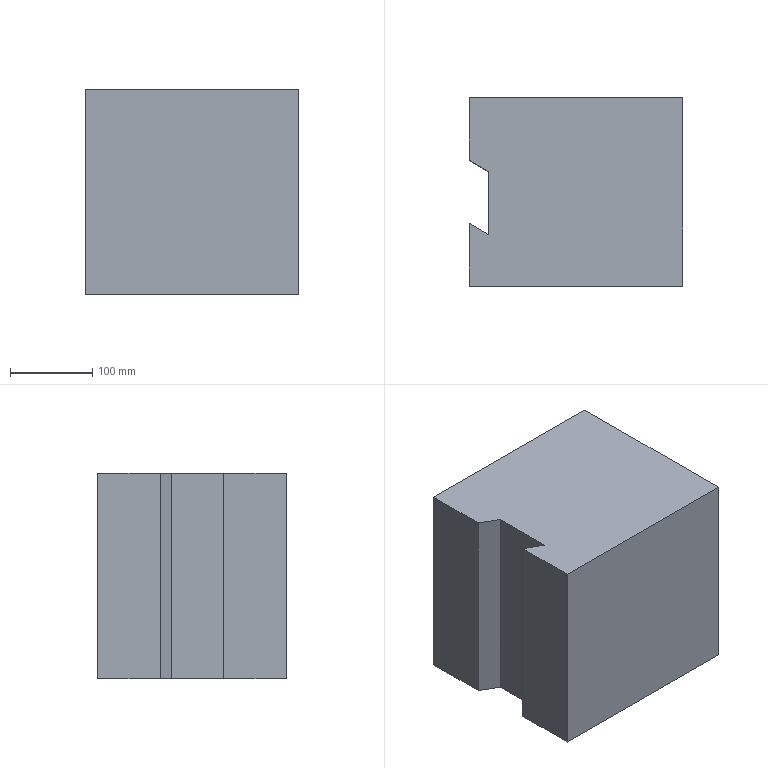Part | STEP file | Printer | 1 solid | 10 faces | box 260 x 230 x 250 mm | volume 14489193 mm3 | plane 10
STEP:
#1=CARTESIAN_POINT('',(0.,0.,0.));
#2=DIRECTION('',(0.,0.,1.));
#3=DIRECTION('',(1.,0.,0.));
#4=AXIS2_PLACEMENT_3D('',#1,#2,#3);
#5=CARTESIAN_POINT('',(-130.,115.,125.));
#6=VERTEX_POINT('',#5);
#7=CARTESIAN_POINT('',(-130.,115.,-125.));
#8=VERTEX_POINT('',#7);
#9=CARTESIAN_POINT('',(-130.,115.,125.));
#10=DIRECTION('',(0.,0.,-1.));
#11=VECTOR('',#10,1.);
#12=LINE('',#9,#11);
#13=CARTESIAN_POINT('',(-130.,115.,125.));
#14=DIRECTION('',(0.,-1.,0.));
#15=DIRECTION('',(0.,0.,-1.));
#16=AXIS2_PLACEMENT_3D('',#13,#14,#15);
#17=PLANE('',#16);
#18=CARTESIAN_POINT('',(0.,0.));
#19=DIRECTION('',(1.,0.));
#20=VECTOR('',#19,1.);
#21=LINE('',#18,#20);
#22=(GEOMETRIC_REPRESENTATION_CONTEXT(2)PARAMETRIC_REPRESENTATION_CONTEXT()REPRESENTATION_CONTEXT('',''));
#23=DEFINITIONAL_REPRESENTATION('',(#21),#22);
#24=PCURVE('',#17,#23);
#25=CARTESIAN_POINT('',(-130.,115.,125.));
#26=DIRECTION('',(1.,0.,0.));
#27=DIRECTION('',(0.,0.,-1.));
#28=AXIS2_PLACEMENT_3D('',#25,#26,#27);
#29=PLANE('',#28);
#30=CARTESIAN_POINT('',(0.,0.));
#31=DIRECTION('',(1.,0.));
#32=VECTOR('',#31,1.);
#33=LINE('',#30,#32);
#34=(GEOMETRIC_REPRESENTATION_CONTEXT(2)PARAMETRIC_REPRESENTATION_CONTEXT()REPRESENTATION_CONTEXT('',''));
#35=DEFINITIONAL_REPRESENTATION('',(#33),#34);
#36=PCURVE('',#29,#35);
#37=SURFACE_CURVE('',#12,(#24,#36),.PCURVE_S1.);
#38=EDGE_CURVE('',#6,#8,#37,.T.);
#39=ORIENTED_EDGE('',*,*,#38,.F.);
#40=CARTESIAN_POINT('',(130.,115.,125.));
#41=VERTEX_POINT('',#40);
#42=CARTESIAN_POINT('',(-130.,115.,125.));
#43=DIRECTION('',(-1.,0.,0.));
#44=VECTOR('',#43,1.);
#45=LINE('',#42,#44);
#46=CARTESIAN_POINT('',(0.,0.));
#47=DIRECTION('',(0.,-1.));
#48=VECTOR('',#47,1.);
#49=LINE('',#46,#48);
#50=(GEOMETRIC_REPRESENTATION_CONTEXT(2)PARAMETRIC_REPRESENTATION_CONTEXT()REPRESENTATION_CONTEXT('',''));
#51=DEFINITIONAL_REPRESENTATION('',(#49),#50);
#52=PCURVE('',#17,#51);
#53=CARTESIAN_POINT('',(130.,-115.,125.));
#54=DIRECTION('',(0.,0.,1.));
#55=DIRECTION('',(1.,0.,0.));
#56=AXIS2_PLACEMENT_3D('',#53,#54,#55);
#57=PLANE('',#56);
#58=CARTESIAN_POINT('',(-260.,230.));
#59=DIRECTION('',(-1.,0.));
#60=VECTOR('',#59,1.);
#61=LINE('',#58,#60);
#62=(GEOMETRIC_REPRESENTATION_CONTEXT(2)PARAMETRIC_REPRESENTATION_CONTEXT()REPRESENTATION_CONTEXT('',''));
#63=DEFINITIONAL_REPRESENTATION('',(#61),#62);
#64=PCURVE('',#57,#63);
#65=SURFACE_CURVE('',#45,(#52,#64),.PCURVE_S1.);
#66=EDGE_CURVE('',#41,#6,#65,.T.);
#67=ORIENTED_EDGE('',*,*,#66,.F.);
#68=CARTESIAN_POINT('',(130.,115.,-125.));
#69=VERTEX_POINT('',#68);
#70=CARTESIAN_POINT('',(130.,115.,125.));
#71=DIRECTION('',(0.,0.,1.));
#72=VECTOR('',#71,1.);
#73=LINE('',#70,#72);
#74=CARTESIAN_POINT('',(0.,260.));
#75=DIRECTION('',(-1.,0.));
#76=VECTOR('',#75,1.);
#77=LINE('',#74,#76);
#78=(GEOMETRIC_REPRESENTATION_CONTEXT(2)PARAMETRIC_REPRESENTATION_CONTEXT()REPRESENTATION_CONTEXT('',''));
#79=DEFINITIONAL_REPRESENTATION('',(#77),#78);
#80=PCURVE('',#17,#79);
#81=CARTESIAN_POINT('',(130.,115.,125.));
#82=DIRECTION('',(-1.,0.,0.));
#83=DIRECTION('',(0.,0.,1.));
#84=AXIS2_PLACEMENT_3D('',#81,#82,#83);
#85=PLANE('',#84);
#86=CARTESIAN_POINT('',(0.,0.));
#87=DIRECTION('',(1.,0.));
#88=VECTOR('',#87,1.);
#89=LINE('',#86,#88);
#90=(GEOMETRIC_REPRESENTATION_CONTEXT(2)PARAMETRIC_REPRESENTATION_CONTEXT()REPRESENTATION_CONTEXT('',''));
#91=DEFINITIONAL_REPRESENTATION('',(#89),#90);
#92=PCURVE('',#85,#91);
#93=SURFACE_CURVE('',#73,(#80,#92),.PCURVE_S1.);
#94=EDGE_CURVE('',#69,#41,#93,.T.);
#95=ORIENTED_EDGE('',*,*,#94,.F.);
#96=CARTESIAN_POINT('',(-130.,115.,-125.));
#97=DIRECTION('',(1.,0.,0.));
#98=VECTOR('',#97,1.);
#99=LINE('',#96,#98);
#100=CARTESIAN_POINT('',(250.,0.));
#101=DIRECTION('',(0.,1.));
#102=VECTOR('',#101,1.);
#103=LINE('',#100,#102);
#104=(GEOMETRIC_REPRESENTATION_CONTEXT(2)PARAMETRIC_REPRESENTATION_CONTEXT()REPRESENTATION_CONTEXT('',''));
#105=DEFINITIONAL_REPRESENTATION('',(#103),#104);
#106=PCURVE('',#17,#105);
#107=CARTESIAN_POINT('',(130.,-115.,-125.));
#108=DIRECTION('',(0.,0.,1.));
#109=DIRECTION('',(1.,0.,0.));
#110=AXIS2_PLACEMENT_3D('',#107,#108,#109);
#111=PLANE('',#110);
#112=CARTESIAN_POINT('',(-260.,230.));
#113=DIRECTION('',(1.,0.));
#114=VECTOR('',#113,1.);
#115=LINE('',#112,#114);
#116=(GEOMETRIC_REPRESENTATION_CONTEXT(2)PARAMETRIC_REPRESENTATION_CONTEXT()REPRESENTATION_CONTEXT('',''));
#117=DEFINITIONAL_REPRESENTATION('',(#115),#116);
#118=PCURVE('',#111,#117);
#119=SURFACE_CURVE('',#99,(#106,#118),.PCURVE_S1.);
#120=EDGE_CURVE('',#8,#69,#119,.T.);
#121=ORIENTED_EDGE('',*,*,#120,.F.);
#122=EDGE_LOOP('',(#39,#67,#95,#121));
#123=FACE_BOUND('',#122,.T.);
#124=ADVANCED_FACE('',(#123),#17,.F.);
#125=CARTESIAN_POINT('',(-130.,-115.,-125.));
#126=VERTEX_POINT('',#125);
#127=CARTESIAN_POINT('',(130.,-115.,-125.));
#128=VERTEX_POINT('',#127);
#129=CARTESIAN_POINT('',(130.,-115.,-125.));
#130=DIRECTION('',(1.,0.,0.));
#131=VECTOR('',#130,1.);
#132=LINE('',#129,#131);
#133=CARTESIAN_POINT('',(0.,0.));
#134=DIRECTION('',(1.,0.));
#135=VECTOR('',#134,1.);
#136=LINE('',#133,#135);
#137=(GEOMETRIC_REPRESENTATION_CONTEXT(2)PARAMETRIC_REPRESENTATION_CONTEXT()REPRESENTATION_CONTEXT('',''));
#138=DEFINITIONAL_REPRESENTATION('',(#136),#137);
#139=PCURVE('',#111,#138);
#140=CARTESIAN_POINT('',(-130.,-115.,125.));
#141=DIRECTION('',(0.,1.,0.));
#142=DIRECTION('',(0.,0.,1.));
#143=AXIS2_PLACEMENT_3D('',#140,#141,#142);
#144=PLANE('',#143);
#145=CARTESIAN_POINT('',(-250.,260.));
#146=DIRECTION('',(0.,1.));
#147=VECTOR('',#146,1.);
#148=LINE('',#145,#147);
#149=(GEOMETRIC_REPRESENTATION_CONTEXT(2)PARAMETRIC_REPRESENTATION_CONTEXT()REPRESENTATION_CONTEXT('',''));
#150=DEFINITIONAL_REPRESENTATION('',(#148),#149);
#151=PCURVE('',#144,#150);
#152=SURFACE_CURVE('',#132,(#139,#151),.PCURVE_S1.);
#153=EDGE_CURVE('',#126,#128,#152,.T.);
#154=ORIENTED_EDGE('',*,*,#153,.F.);
#155=CARTESIAN_POINT('',(-130.,-38.354,-125.));
#156=VERTEX_POINT('',#155);
#157=CARTESIAN_POINT('',(-130.,-115.,-125.));
#158=DIRECTION('',(0.,-1.,0.));
#159=VECTOR('',#158,1.);
#160=LINE('',#157,#159);
#161=CARTESIAN_POINT('',(-260.,0.));
#162=DIRECTION('',(0.,-1.));
#163=VECTOR('',#162,1.);
#164=LINE('',#161,#163);
#165=(GEOMETRIC_REPRESENTATION_CONTEXT(2)PARAMETRIC_REPRESENTATION_CONTEXT()REPRESENTATION_CONTEXT('',''));
#166=DEFINITIONAL_REPRESENTATION('',(#164),#165);
#167=PCURVE('',#111,#166);
#168=CARTESIAN_POINT('',(-130.,-38.354,125.));
#169=DIRECTION('',(1.,0.,0.));
#170=DIRECTION('',(0.,0.,-1.));
#171=AXIS2_PLACEMENT_3D('',#168,#169,#170);
#172=PLANE('',#171);
#173=CARTESIAN_POINT('',(250.,-76.646));
#174=DIRECTION('',(0.,-1.));
#175=VECTOR('',#174,1.);
#176=LINE('',#173,#175);
#177=(GEOMETRIC_REPRESENTATION_CONTEXT(2)PARAMETRIC_REPRESENTATION_CONTEXT()REPRESENTATION_CONTEXT('',''));
#178=DEFINITIONAL_REPRESENTATION('',(#176),#177);
#179=PCURVE('',#172,#178);
#180=SURFACE_CURVE('',#160,(#167,#179),.PCURVE_S1.);
#181=EDGE_CURVE('',#156,#126,#180,.T.);
#182=ORIENTED_EDGE('',*,*,#181,.F.);
#183=CARTESIAN_POINT('',(-105.971,-52.25,-125.));
#184=VERTEX_POINT('',#183);
#185=CARTESIAN_POINT('',(-105.971,-52.25,-125.));
#186=DIRECTION('',(-0.8657,0.5006,0.));
#187=VECTOR('',#186,1.);
#188=LINE('',#185,#187);
#189=CARTESIAN_POINT('',(-235.971,62.75));
#190=DIRECTION('',(-0.8657,0.5006));
#191=VECTOR('',#190,1.);
#192=LINE('',#189,#191);
#193=(GEOMETRIC_REPRESENTATION_CONTEXT(2)PARAMETRIC_REPRESENTATION_CONTEXT()REPRESENTATION_CONTEXT('',''));
#194=DEFINITIONAL_REPRESENTATION('',(#192),#193);
#195=PCURVE('',#111,#194);
#196=CARTESIAN_POINT('',(-105.971,-52.25,125.));
#197=DIRECTION('',(-0.5006,-0.8657,0.));
#198=DIRECTION('',(0.8657,-0.5006,0.));
#199=AXIS2_PLACEMENT_3D('',#196,#197,#198);
#200=PLANE('',#199);
#201=CARTESIAN_POINT('',(0.,-250.));
#202=DIRECTION('',(-1.,0.));
#203=VECTOR('',#202,1.);
#204=LINE('',#201,#203);
#205=(GEOMETRIC_REPRESENTATION_CONTEXT(2)PARAMETRIC_REPRESENTATION_CONTEXT()REPRESENTATION_CONTEXT('',''));
#206=DEFINITIONAL_REPRESENTATION('',(#204),#205);
#207=PCURVE('',#200,#206);
#208=SURFACE_CURVE('',#188,(#195,#207),.PCURVE_S1.);
#209=EDGE_CURVE('',#184,#156,#208,.T.);
#210=ORIENTED_EDGE('',*,*,#209,.F.);
#211=CARTESIAN_POINT('',(-105.971,24.459,-125.));
#212=VERTEX_POINT('',#211);
#213=CARTESIAN_POINT('',(-105.971,-115.,-125.));
#214=DIRECTION('',(0.,-1.,0.));
#215=VECTOR('',#214,1.);
#216=LINE('',#213,#215);
#217=CARTESIAN_POINT('',(-235.971,0.));
#218=DIRECTION('',(0.,-1.));
#219=VECTOR('',#218,1.);
#220=LINE('',#217,#219);
#221=(GEOMETRIC_REPRESENTATION_CONTEXT(2)PARAMETRIC_REPRESENTATION_CONTEXT()REPRESENTATION_CONTEXT('',''));
#222=DEFINITIONAL_REPRESENTATION('',(#220),#221);
#223=PCURVE('',#111,#222);
#224=CARTESIAN_POINT('',(-105.971,24.459,125.));
#225=DIRECTION('',(1.,0.,0.));
#226=DIRECTION('',(0.,0.,-1.));
#227=AXIS2_PLACEMENT_3D('',#224,#225,#226);
#228=PLANE('',#227);
#229=CARTESIAN_POINT('',(250.,-139.459));
#230=DIRECTION('',(0.,-1.));
#231=VECTOR('',#230,1.);
#232=LINE('',#229,#231);
#233=(GEOMETRIC_REPRESENTATION_CONTEXT(2)PARAMETRIC_REPRESENTATION_CONTEXT()REPRESENTATION_CONTEXT('',''));
#234=DEFINITIONAL_REPRESENTATION('',(#232),#233);
#235=PCURVE('',#228,#234);
#236=SURFACE_CURVE('',#216,(#223,#235),.PCURVE_S1.);
#237=EDGE_CURVE('',#212,#184,#236,.T.);
#238=ORIENTED_EDGE('',*,*,#237,.F.);
#239=CARTESIAN_POINT('',(-130.,38.354,-125.));
#240=VERTEX_POINT('',#239);
#241=CARTESIAN_POINT('',(-130.,38.354,-125.));
#242=DIRECTION('',(0.8657,-0.5006,0.));
#243=VECTOR('',#242,1.);
#244=LINE('',#241,#243);
#245=CARTESIAN_POINT('',(-260.,153.354));
#246=DIRECTION('',(0.8657,-0.5006));
#247=VECTOR('',#246,1.);
#248=LINE('',#245,#247);
#249=(GEOMETRIC_REPRESENTATION_CONTEXT(2)PARAMETRIC_REPRESENTATION_CONTEXT()REPRESENTATION_CONTEXT('',''));
#250=DEFINITIONAL_REPRESENTATION('',(#248),#249);
#251=PCURVE('',#111,#250);
#252=CARTESIAN_POINT('',(-130.,38.354,125.));
#253=DIRECTION('',(0.5006,0.8657,0.));
#254=DIRECTION('',(-0.8657,0.5006,0.));
#255=AXIS2_PLACEMENT_3D('',#252,#253,#254);
#256=PLANE('',#255);
#257=CARTESIAN_POINT('',(0.,-250.));
#258=DIRECTION('',(-1.,0.));
#259=VECTOR('',#258,1.);
#260=LINE('',#257,#259);
#261=(GEOMETRIC_REPRESENTATION_CONTEXT(2)PARAMETRIC_REPRESENTATION_CONTEXT()REPRESENTATION_CONTEXT('',''));
#262=DEFINITIONAL_REPRESENTATION('',(#260),#261);
#263=PCURVE('',#256,#262);
#264=SURFACE_CURVE('',#244,(#251,#263),.PCURVE_S1.);
#265=EDGE_CURVE('',#240,#212,#264,.T.);
#266=ORIENTED_EDGE('',*,*,#265,.F.);
#267=CARTESIAN_POINT('',(-130.,-115.,-125.));
#268=DIRECTION('',(0.,-1.,0.));
#269=VECTOR('',#268,1.);
#270=LINE('',#267,#269);
#271=CARTESIAN_POINT('',(-260.,0.));
#272=DIRECTION('',(0.,-1.));
#273=VECTOR('',#272,1.);
#274=LINE('',#271,#273);
#275=(GEOMETRIC_REPRESENTATION_CONTEXT(2)PARAMETRIC_REPRESENTATION_CONTEXT()REPRESENTATION_CONTEXT('',''));
#276=DEFINITIONAL_REPRESENTATION('',(#274),#275);
#277=PCURVE('',#111,#276);
#278=CARTESIAN_POINT('',(250.,-230.));
#279=DIRECTION('',(0.,-1.));
#280=VECTOR('',#279,1.);
#281=LINE('',#278,#280);
#282=(GEOMETRIC_REPRESENTATION_CONTEXT(2)PARAMETRIC_REPRESENTATION_CONTEXT()REPRESENTATION_CONTEXT('',''));
#283=DEFINITIONAL_REPRESENTATION('',(#281),#282);
#284=PCURVE('',#29,#283);
#285=SURFACE_CURVE('',#270,(#277,#284),.PCURVE_S1.);
#286=EDGE_CURVE('',#8,#240,#285,.T.);
#287=ORIENTED_EDGE('',*,*,#286,.F.);
#288=ORIENTED_EDGE('',*,*,#120,.T.);
#289=CARTESIAN_POINT('',(130.,-115.,-125.));
#290=DIRECTION('',(0.,1.,0.));
#291=VECTOR('',#290,1.);
#292=LINE('',#289,#291);
#293=CARTESIAN_POINT('',(0.,0.));
#294=DIRECTION('',(0.,1.));
#295=VECTOR('',#294,1.);
#296=LINE('',#293,#295);
#297=(GEOMETRIC_REPRESENTATION_CONTEXT(2)PARAMETRIC_REPRESENTATION_CONTEXT()REPRESENTATION_CONTEXT('',''));
#298=DEFINITIONAL_REPRESENTATION('',(#296),#297);
#299=PCURVE('',#111,#298);
#300=CARTESIAN_POINT('',(-250.,-230.));
#301=DIRECTION('',(0.,1.));
#302=VECTOR('',#301,1.);
#303=LINE('',#300,#302);
#304=(GEOMETRIC_REPRESENTATION_CONTEXT(2)PARAMETRIC_REPRESENTATION_CONTEXT()REPRESENTATION_CONTEXT('',''));
#305=DEFINITIONAL_REPRESENTATION('',(#303),#304);
#306=PCURVE('',#85,#305);
#307=SURFACE_CURVE('',#292,(#299,#306),.PCURVE_S1.);
#308=EDGE_CURVE('',#128,#69,#307,.T.);
#309=ORIENTED_EDGE('',*,*,#308,.F.);
#310=EDGE_LOOP('',(#154,#182,#210,#238,#266,#287,#288,#309));
#311=FACE_BOUND('',#310,.T.);
#312=ADVANCED_FACE('',(#311),#111,.F.);
#313=CARTESIAN_POINT('',(-130.,38.354,125.));
#314=VERTEX_POINT('',#313);
#315=CARTESIAN_POINT('',(-130.,38.354,125.));
#316=DIRECTION('',(0.,0.,-1.));
#317=VECTOR('',#316,1.);
#318=LINE('',#315,#317);
#319=CARTESIAN_POINT('',(0.,-76.646));
#320=DIRECTION('',(1.,0.));
#321=VECTOR('',#320,1.);
#322=LINE('',#319,#321);
#323=(GEOMETRIC_REPRESENTATION_CONTEXT(2)PARAMETRIC_REPRESENTATION_CONTEXT()REPRESENTATION_CONTEXT('',''));
#324=DEFINITIONAL_REPRESENTATION('',(#322),#323);
#325=PCURVE('',#29,#324);
#326=CARTESIAN_POINT('',(0.,0.));
#327=DIRECTION('',(0.,-1.));
#328=VECTOR('',#327,1.);
#329=LINE('',#326,#328);
#330=(GEOMETRIC_REPRESENTATION_CONTEXT(2)PARAMETRIC_REPRESENTATION_CONTEXT()REPRESENTATION_CONTEXT('',''));
#331=DEFINITIONAL_REPRESENTATION('',(#329),#330);
#332=PCURVE('',#256,#331);
#333=SURFACE_CURVE('',#318,(#325,#332),.PCURVE_S1.);
#334=EDGE_CURVE('',#314,#240,#333,.T.);
#335=ORIENTED_EDGE('',*,*,#334,.F.);
#336=CARTESIAN_POINT('',(-130.,115.,125.));
#337=DIRECTION('',(0.,-1.,0.));
#338=VECTOR('',#337,1.);
#339=LINE('',#336,#338);
#340=CARTESIAN_POINT('',(0.,0.));
#341=DIRECTION('',(0.,-1.));
#342=VECTOR('',#341,1.);
#343=LINE('',#340,#342);
#344=(GEOMETRIC_REPRESENTATION_CONTEXT(2)PARAMETRIC_REPRESENTATION_CONTEXT()REPRESENTATION_CONTEXT('',''));
#345=DEFINITIONAL_REPRESENTATION('',(#343),#344);
#346=PCURVE('',#29,#345);
#347=CARTESIAN_POINT('',(-260.,230.));
#348=DIRECTION('',(0.,-1.));
#349=VECTOR('',#348,1.);
#350=LINE('',#347,#349);
#351=(GEOMETRIC_REPRESENTATION_CONTEXT(2)PARAMETRIC_REPRESENTATION_CONTEXT()REPRESENTATION_CONTEXT('',''));
#352=DEFINITIONAL_REPRESENTATION('',(#350),#351);
#353=PCURVE('',#57,#352);
#354=SURFACE_CURVE('',#339,(#346,#353),.PCURVE_S1.);
#355=EDGE_CURVE('',#6,#314,#354,.T.);
#356=ORIENTED_EDGE('',*,*,#355,.F.);
#357=ORIENTED_EDGE('',*,*,#38,.T.);
#358=ORIENTED_EDGE('',*,*,#286,.T.);
#359=EDGE_LOOP('',(#335,#356,#357,#358));
#360=FACE_BOUND('',#359,.T.);
#361=ADVANCED_FACE('',(#360),#29,.F.);
#362=CARTESIAN_POINT('',(-130.,-38.354,125.));
#363=VERTEX_POINT('',#362);
#364=CARTESIAN_POINT('',(-130.,-115.,125.));
#365=VERTEX_POINT('',#364);
#366=CARTESIAN_POINT('',(-130.,-115.,125.));
#367=DIRECTION('',(0.,-1.,0.));
#368=VECTOR('',#367,1.);
#369=LINE('',#366,#368);
#370=CARTESIAN_POINT('',(-260.,0.));
#371=DIRECTION('',(0.,-1.));
#372=VECTOR('',#371,1.);
#373=LINE('',#370,#372);
#374=(GEOMETRIC_REPRESENTATION_CONTEXT(2)PARAMETRIC_REPRESENTATION_CONTEXT()REPRESENTATION_CONTEXT('',''));
#375=DEFINITIONAL_REPRESENTATION('',(#373),#374);
#376=PCURVE('',#57,#375);
#377=CARTESIAN_POINT('',(0.,-76.646));
#378=DIRECTION('',(0.,-1.));
#379=VECTOR('',#378,1.);
#380=LINE('',#377,#379);
#381=(GEOMETRIC_REPRESENTATION_CONTEXT(2)PARAMETRIC_REPRESENTATION_CONTEXT()REPRESENTATION_CONTEXT('',''));
#382=DEFINITIONAL_REPRESENTATION('',(#380),#381);
#383=PCURVE('',#172,#382);
#384=SURFACE_CURVE('',#369,(#376,#383),.PCURVE_S1.);
#385=EDGE_CURVE('',#363,#365,#384,.T.);
#386=ORIENTED_EDGE('',*,*,#385,.T.);
#387=CARTESIAN_POINT('',(130.,-115.,125.));
#388=VERTEX_POINT('',#387);
#389=CARTESIAN_POINT('',(130.,-115.,125.));
#390=DIRECTION('',(1.,0.,0.));
#391=VECTOR('',#390,1.);
#392=LINE('',#389,#391);
#393=CARTESIAN_POINT('',(0.,0.));
#394=DIRECTION('',(1.,0.));
#395=VECTOR('',#394,1.);
#396=LINE('',#393,#395);
#397=(GEOMETRIC_REPRESENTATION_CONTEXT(2)PARAMETRIC_REPRESENTATION_CONTEXT()REPRESENTATION_CONTEXT('',''));
#398=DEFINITIONAL_REPRESENTATION('',(#396),#397);
#399=PCURVE('',#57,#398);
#400=CARTESIAN_POINT('',(0.,260.));
#401=DIRECTION('',(0.,1.));
#402=VECTOR('',#401,1.);
#403=LINE('',#400,#402);
#404=(GEOMETRIC_REPRESENTATION_CONTEXT(2)PARAMETRIC_REPRESENTATION_CONTEXT()REPRESENTATION_CONTEXT('',''));
#405=DEFINITIONAL_REPRESENTATION('',(#403),#404);
#406=PCURVE('',#144,#405);
#407=SURFACE_CURVE('',#392,(#399,#406),.PCURVE_S1.);
#408=EDGE_CURVE('',#365,#388,#407,.T.);
#409=ORIENTED_EDGE('',*,*,#408,.T.);
#410=CARTESIAN_POINT('',(130.,-115.,125.));
#411=DIRECTION('',(0.,1.,0.));
#412=VECTOR('',#411,1.);
#413=LINE('',#410,#412);
#414=CARTESIAN_POINT('',(0.,0.));
#415=DIRECTION('',(0.,1.));
#416=VECTOR('',#415,1.);
#417=LINE('',#414,#416);
#418=(GEOMETRIC_REPRESENTATION_CONTEXT(2)PARAMETRIC_REPRESENTATION_CONTEXT()REPRESENTATION_CONTEXT('',''));
#419=DEFINITIONAL_REPRESENTATION('',(#417),#418);
#420=PCURVE('',#57,#419);
#421=CARTESIAN_POINT('',(0.,-230.));
#422=DIRECTION('',(0.,1.));
#423=VECTOR('',#422,1.);
#424=LINE('',#421,#423);
#425=(GEOMETRIC_REPRESENTATION_CONTEXT(2)PARAMETRIC_REPRESENTATION_CONTEXT()REPRESENTATION_CONTEXT('',''));
#426=DEFINITIONAL_REPRESENTATION('',(#424),#425);
#427=PCURVE('',#85,#426);
#428=SURFACE_CURVE('',#413,(#420,#427),.PCURVE_S1.);
#429=EDGE_CURVE('',#388,#41,#428,.T.);
#430=ORIENTED_EDGE('',*,*,#429,.T.);
#431=ORIENTED_EDGE('',*,*,#66,.T.);
#432=ORIENTED_EDGE('',*,*,#355,.T.);
#433=CARTESIAN_POINT('',(-105.971,24.459,125.));
#434=VERTEX_POINT('',#433);
#435=CARTESIAN_POINT('',(-130.,38.354,125.));
#436=DIRECTION('',(0.8657,-0.5006,0.));
#437=VECTOR('',#436,1.);
#438=LINE('',#435,#437);
#439=CARTESIAN_POINT('',(-260.,153.354));
#440=DIRECTION('',(0.8657,-0.5006));
#441=VECTOR('',#440,1.);
#442=LINE('',#439,#441);
#443=(GEOMETRIC_REPRESENTATION_CONTEXT(2)PARAMETRIC_REPRESENTATION_CONTEXT()REPRESENTATION_CONTEXT('',''));
#444=DEFINITIONAL_REPRESENTATION('',(#442),#443);
#445=PCURVE('',#57,#444);
#446=CARTESIAN_POINT('',(0.,0.));
#447=DIRECTION('',(-1.,0.));
#448=VECTOR('',#447,1.);
#449=LINE('',#446,#448);
#450=(GEOMETRIC_REPRESENTATION_CONTEXT(2)PARAMETRIC_REPRESENTATION_CONTEXT()REPRESENTATION_CONTEXT('',''));
#451=DEFINITIONAL_REPRESENTATION('',(#449),#450);
#452=PCURVE('',#256,#451);
#453=SURFACE_CURVE('',#438,(#445,#452),.PCURVE_S1.);
#454=EDGE_CURVE('',#314,#434,#453,.T.);
#455=ORIENTED_EDGE('',*,*,#454,.T.);
#456=CARTESIAN_POINT('',(-105.971,-52.25,125.));
#457=VERTEX_POINT('',#456);
#458=CARTESIAN_POINT('',(-105.971,-115.,125.));
#459=DIRECTION('',(0.,-1.,0.));
#460=VECTOR('',#459,1.);
#461=LINE('',#458,#460);
#462=CARTESIAN_POINT('',(-235.971,0.));
#463=DIRECTION('',(0.,-1.));
#464=VECTOR('',#463,1.);
#465=LINE('',#462,#464);
#466=(GEOMETRIC_REPRESENTATION_CONTEXT(2)PARAMETRIC_REPRESENTATION_CONTEXT()REPRESENTATION_CONTEXT('',''));
#467=DEFINITIONAL_REPRESENTATION('',(#465),#466);
#468=PCURVE('',#57,#467);
#469=CARTESIAN_POINT('',(0.,-139.459));
#470=DIRECTION('',(0.,-1.));
#471=VECTOR('',#470,1.);
#472=LINE('',#469,#471);
#473=(GEOMETRIC_REPRESENTATION_CONTEXT(2)PARAMETRIC_REPRESENTATION_CONTEXT()REPRESENTATION_CONTEXT('',''));
#474=DEFINITIONAL_REPRESENTATION('',(#472),#473);
#475=PCURVE('',#228,#474);
#476=SURFACE_CURVE('',#461,(#468,#475),.PCURVE_S1.);
#477=EDGE_CURVE('',#434,#457,#476,.T.);
#478=ORIENTED_EDGE('',*,*,#477,.T.);
#479=CARTESIAN_POINT('',(-105.971,-52.25,125.));
#480=DIRECTION('',(-0.8657,0.5006,0.));
#481=VECTOR('',#480,1.);
#482=LINE('',#479,#481);
#483=CARTESIAN_POINT('',(-235.971,62.75));
#484=DIRECTION('',(-0.8657,0.5006));
#485=VECTOR('',#484,1.);
#486=LINE('',#483,#485);
#487=(GEOMETRIC_REPRESENTATION_CONTEXT(2)PARAMETRIC_REPRESENTATION_CONTEXT()REPRESENTATION_CONTEXT('',''));
#488=DEFINITIONAL_REPRESENTATION('',(#486),#487);
#489=PCURVE('',#57,#488);
#490=CARTESIAN_POINT('',(0.,0.));
#491=DIRECTION('',(-1.,0.));
#492=VECTOR('',#491,1.);
#493=LINE('',#490,#492);
#494=(GEOMETRIC_REPRESENTATION_CONTEXT(2)PARAMETRIC_REPRESENTATION_CONTEXT()REPRESENTATION_CONTEXT('',''));
#495=DEFINITIONAL_REPRESENTATION('',(#493),#494);
#496=PCURVE('',#200,#495);
#497=SURFACE_CURVE('',#482,(#489,#496),.PCURVE_S1.);
#498=EDGE_CURVE('',#457,#363,#497,.T.);
#499=ORIENTED_EDGE('',*,*,#498,.T.);
#500=EDGE_LOOP('',(#386,#409,#430,#431,#432,#455,#478,#499));
#501=FACE_BOUND('',#500,.T.);
#502=ADVANCED_FACE('',(#501),#57,.T.);
#503=ORIENTED_EDGE('',*,*,#94,.T.);
#504=ORIENTED_EDGE('',*,*,#429,.F.);
#505=CARTESIAN_POINT('',(130.,-115.,125.));
#506=DIRECTION('',(0.,0.,1.));
#507=VECTOR('',#506,1.);
#508=LINE('',#505,#507);
#509=CARTESIAN_POINT('',(0.,-230.));
#510=DIRECTION('',(1.,0.));
#511=VECTOR('',#510,1.);
#512=LINE('',#509,#511);
#513=(GEOMETRIC_REPRESENTATION_CONTEXT(2)PARAMETRIC_REPRESENTATION_CONTEXT()REPRESENTATION_CONTEXT('',''));
#514=DEFINITIONAL_REPRESENTATION('',(#512),#513);
#515=PCURVE('',#85,#514);
#516=CARTESIAN_POINT('',(0.,260.));
#517=DIRECTION('',(1.,0.));
#518=VECTOR('',#517,1.);
#519=LINE('',#516,#518);
#520=(GEOMETRIC_REPRESENTATION_CONTEXT(2)PARAMETRIC_REPRESENTATION_CONTEXT()REPRESENTATION_CONTEXT('',''));
#521=DEFINITIONAL_REPRESENTATION('',(#519),#520);
#522=PCURVE('',#144,#521);
#523=SURFACE_CURVE('',#508,(#515,#522),.PCURVE_S1.);
#524=EDGE_CURVE('',#128,#388,#523,.T.);
#525=ORIENTED_EDGE('',*,*,#524,.F.);
#526=ORIENTED_EDGE('',*,*,#308,.T.);
#527=EDGE_LOOP('',(#503,#504,#525,#526));
#528=FACE_BOUND('',#527,.T.);
#529=ADVANCED_FACE('',(#528),#85,.F.);
#530=ORIENTED_EDGE('',*,*,#524,.T.);
#531=ORIENTED_EDGE('',*,*,#408,.F.);
#532=CARTESIAN_POINT('',(-130.,-115.,125.));
#533=DIRECTION('',(0.,0.,1.));
#534=VECTOR('',#533,1.);
#535=LINE('',#532,#534);
#536=CARTESIAN_POINT('',(0.,0.));
#537=DIRECTION('',(1.,0.));
#538=VECTOR('',#537,1.);
#539=LINE('',#536,#538);
#540=(GEOMETRIC_REPRESENTATION_CONTEXT(2)PARAMETRIC_REPRESENTATION_CONTEXT()REPRESENTATION_CONTEXT('',''));
#541=DEFINITIONAL_REPRESENTATION('',(#539),#540);
#542=PCURVE('',#144,#541);
#543=CARTESIAN_POINT('',(0.,-76.646));
#544=DIRECTION('',(-1.,0.));
#545=VECTOR('',#544,1.);
#546=LINE('',#543,#545);
#547=(GEOMETRIC_REPRESENTATION_CONTEXT(2)PARAMETRIC_REPRESENTATION_CONTEXT()REPRESENTATION_CONTEXT('',''));
#548=DEFINITIONAL_REPRESENTATION('',(#546),#547);
#549=PCURVE('',#172,#548);
#550=SURFACE_CURVE('',#535,(#542,#549),.PCURVE_S1.);
#551=EDGE_CURVE('',#126,#365,#550,.T.);
#552=ORIENTED_EDGE('',*,*,#551,.F.);
#553=ORIENTED_EDGE('',*,*,#153,.T.);
#554=EDGE_LOOP('',(#530,#531,#552,#553));
#555=FACE_BOUND('',#554,.T.);
#556=ADVANCED_FACE('',(#555),#144,.F.);
#557=ORIENTED_EDGE('',*,*,#551,.T.);
#558=ORIENTED_EDGE('',*,*,#385,.F.);
#559=CARTESIAN_POINT('',(-130.,-38.354,125.));
#560=DIRECTION('',(0.,0.,1.));
#561=VECTOR('',#560,1.);
#562=LINE('',#559,#561);
#563=CARTESIAN_POINT('',(0.,0.));
#564=DIRECTION('',(-1.,0.));
#565=VECTOR('',#564,1.);
#566=LINE('',#563,#565);
#567=(GEOMETRIC_REPRESENTATION_CONTEXT(2)PARAMETRIC_REPRESENTATION_CONTEXT()REPRESENTATION_CONTEXT('',''));
#568=DEFINITIONAL_REPRESENTATION('',(#566),#567);
#569=PCURVE('',#172,#568);
#570=CARTESIAN_POINT('',(-27.758,0.));
#571=DIRECTION('',(0.,1.));
#572=VECTOR('',#571,1.);
#573=LINE('',#570,#572);
#574=(GEOMETRIC_REPRESENTATION_CONTEXT(2)PARAMETRIC_REPRESENTATION_CONTEXT()REPRESENTATION_CONTEXT('',''));
#575=DEFINITIONAL_REPRESENTATION('',(#573),#574);
#576=PCURVE('',#200,#575);
#577=SURFACE_CURVE('',#562,(#569,#576),.PCURVE_S1.);
#578=EDGE_CURVE('',#156,#363,#577,.T.);
#579=ORIENTED_EDGE('',*,*,#578,.F.);
#580=ORIENTED_EDGE('',*,*,#181,.T.);
#581=EDGE_LOOP('',(#557,#558,#579,#580));
#582=FACE_BOUND('',#581,.T.);
#583=ADVANCED_FACE('',(#582),#172,.F.);
#584=ORIENTED_EDGE('',*,*,#578,.T.);
#585=ORIENTED_EDGE('',*,*,#498,.F.);
#586=CARTESIAN_POINT('',(-105.971,-52.25,125.));
#587=DIRECTION('',(0.,0.,1.));
#588=VECTOR('',#587,1.);
#589=LINE('',#586,#588);
#590=CARTESIAN_POINT('',(0.,0.));
#591=DIRECTION('',(0.,1.));
#592=VECTOR('',#591,1.);
#593=LINE('',#590,#592);
#594=(GEOMETRIC_REPRESENTATION_CONTEXT(2)PARAMETRIC_REPRESENTATION_CONTEXT()REPRESENTATION_CONTEXT('',''));
#595=DEFINITIONAL_REPRESENTATION('',(#593),#594);
#596=PCURVE('',#200,#595);
#597=CARTESIAN_POINT('',(0.,-76.709));
#598=DIRECTION('',(-1.,0.));
#599=VECTOR('',#598,1.);
#600=LINE('',#597,#599);
#601=(GEOMETRIC_REPRESENTATION_CONTEXT(2)PARAMETRIC_REPRESENTATION_CONTEXT()REPRESENTATION_CONTEXT('',''));
#602=DEFINITIONAL_REPRESENTATION('',(#600),#601);
#603=PCURVE('',#228,#602);
#604=SURFACE_CURVE('',#589,(#596,#603),.PCURVE_S1.);
#605=EDGE_CURVE('',#184,#457,#604,.T.);
#606=ORIENTED_EDGE('',*,*,#605,.F.);
#607=ORIENTED_EDGE('',*,*,#209,.T.);
#608=EDGE_LOOP('',(#584,#585,#606,#607));
#609=FACE_BOUND('',#608,.T.);
#610=ADVANCED_FACE('',(#609),#200,.F.);
#611=ORIENTED_EDGE('',*,*,#605,.T.);
#612=ORIENTED_EDGE('',*,*,#477,.F.);
#613=CARTESIAN_POINT('',(-105.971,24.459,125.));
#614=DIRECTION('',(0.,0.,1.));
#615=VECTOR('',#614,1.);
#616=LINE('',#613,#615);
#617=CARTESIAN_POINT('',(0.,0.));
#618=DIRECTION('',(-1.,0.));
#619=VECTOR('',#618,1.);
#620=LINE('',#617,#619);
#621=(GEOMETRIC_REPRESENTATION_CONTEXT(2)PARAMETRIC_REPRESENTATION_CONTEXT()REPRESENTATION_CONTEXT('',''));
#622=DEFINITIONAL_REPRESENTATION('',(#620),#621);
#623=PCURVE('',#228,#622);
#624=CARTESIAN_POINT('',(-27.758,0.));
#625=DIRECTION('',(0.,1.));
#626=VECTOR('',#625,1.);
#627=LINE('',#624,#626);
#628=(GEOMETRIC_REPRESENTATION_CONTEXT(2)PARAMETRIC_REPRESENTATION_CONTEXT()REPRESENTATION_CONTEXT('',''));
#629=DEFINITIONAL_REPRESENTATION('',(#627),#628);
#630=PCURVE('',#256,#629);
#631=SURFACE_CURVE('',#616,(#623,#630),.PCURVE_S1.);
#632=EDGE_CURVE('',#212,#434,#631,.T.);
#633=ORIENTED_EDGE('',*,*,#632,.F.);
#634=ORIENTED_EDGE('',*,*,#237,.T.);
#635=EDGE_LOOP('',(#611,#612,#633,#634));
#636=FACE_BOUND('',#635,.T.);
#637=ADVANCED_FACE('',(#636),#228,.F.);
#638=ORIENTED_EDGE('',*,*,#632,.T.);
#639=ORIENTED_EDGE('',*,*,#454,.F.);
#640=ORIENTED_EDGE('',*,*,#334,.T.);
#641=ORIENTED_EDGE('',*,*,#265,.T.);
#642=EDGE_LOOP('',(#638,#639,#640,#641));
#643=FACE_BOUND('',#642,.T.);
#644=ADVANCED_FACE('',(#643),#256,.F.);
#645=CLOSED_SHELL('',(#124,#312,#361,#502,#529,#556,#583,#610,#637,#644));
#646=MANIFOLD_SOLID_BREP('',#645);
#647=(LENGTH_UNIT()NAMED_UNIT(*)SI_UNIT(.MILLI.,.METRE.));
#648=UNCERTAINTY_MEASURE_WITH_UNIT(LENGTH_MEASURE(0.0000001),#647,'','');
#649=(NAMED_UNIT(*)PLANE_ANGLE_UNIT()SI_UNIT($,.RADIAN.));
#650=(NAMED_UNIT(*)SI_UNIT($,.STERADIAN.)SOLID_ANGLE_UNIT());
#651=(GEOMETRIC_REPRESENTATION_CONTEXT(3)GLOBAL_UNCERTAINTY_ASSIGNED_CONTEXT((#648))GLOBAL_UNIT_ASSIGNED_CONTEXT((#647,#649,#650))REPRESENTATION_CONTEXT('',''));
#652=ADVANCED_BREP_SHAPE_REPRESENTATION('',(#4,#646),#651);